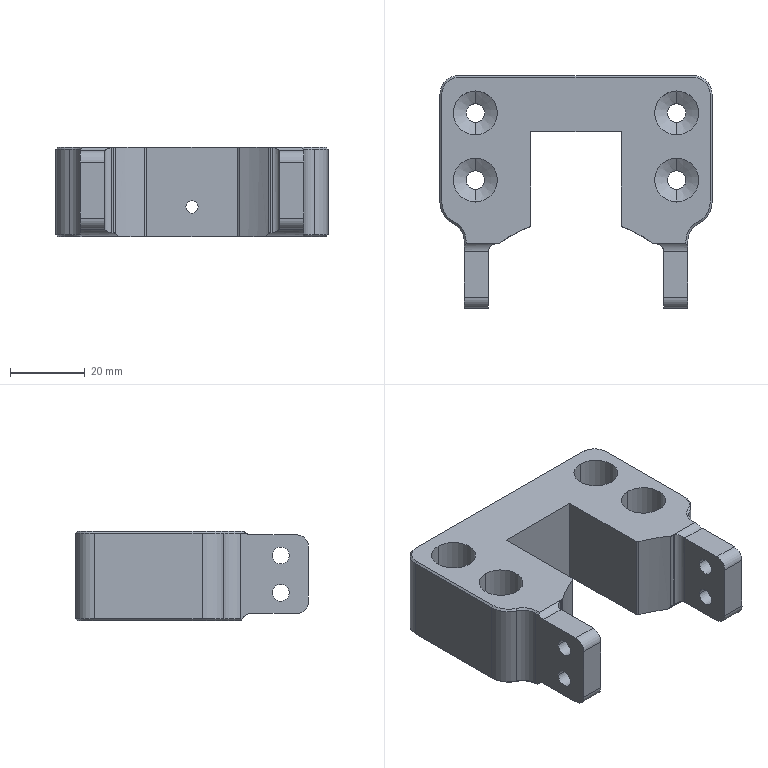Part | 1 solid | 101 faces | box 73 x 62.4 x 24 mm | volume 54741 mm3 | cylinder 50 | plane 31 | cone 20 | commonest cylinder face diameters 6 x10 4.5 x8 5 x8 11.8 x8 2 x4 10 x4